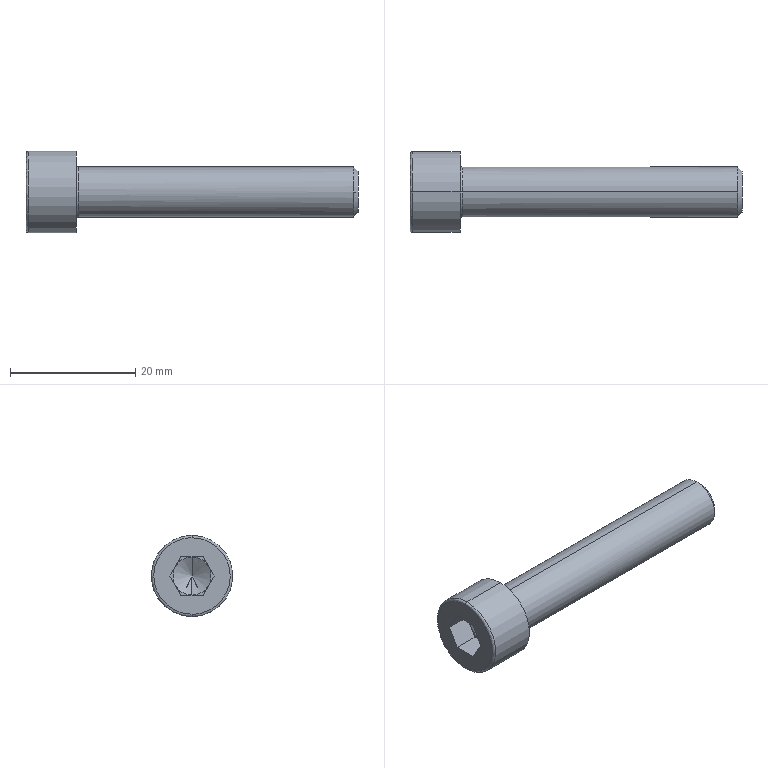Part | STEP file | 0229_312_M8x45 | 1 solid | 27 faces | box 53 x 13 x 13 mm | volume 3172 mm3 | plane 15 | spline 4 | cylinder 4 | cone 4 | commonest cylinder face diameters 8 x2 13 x2